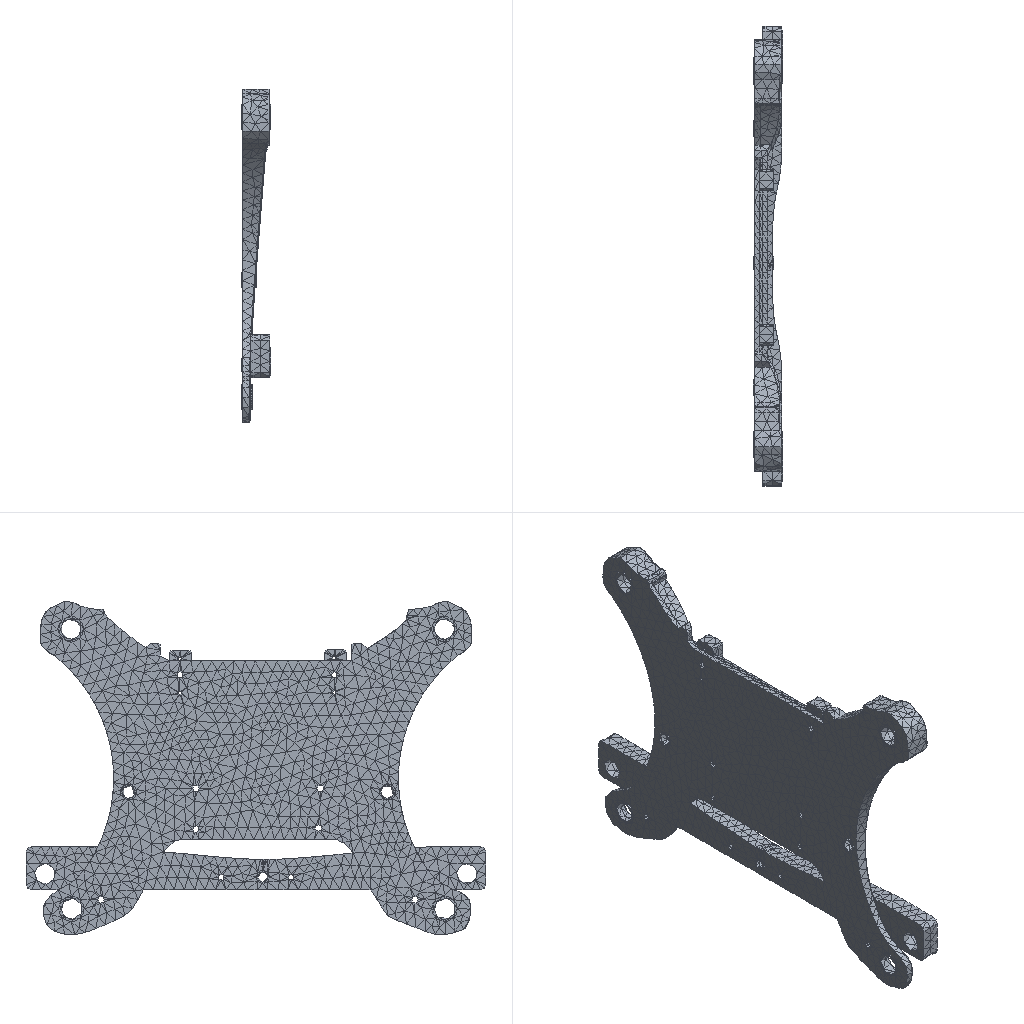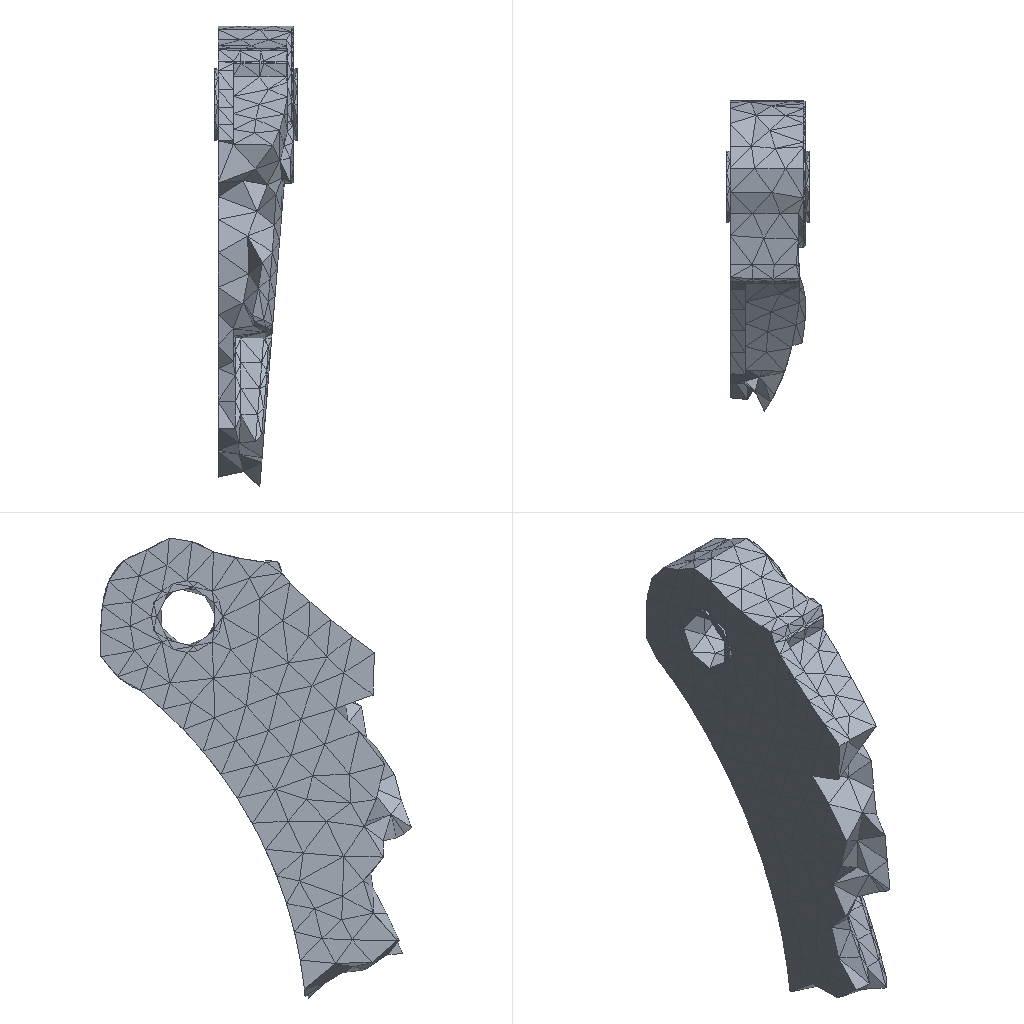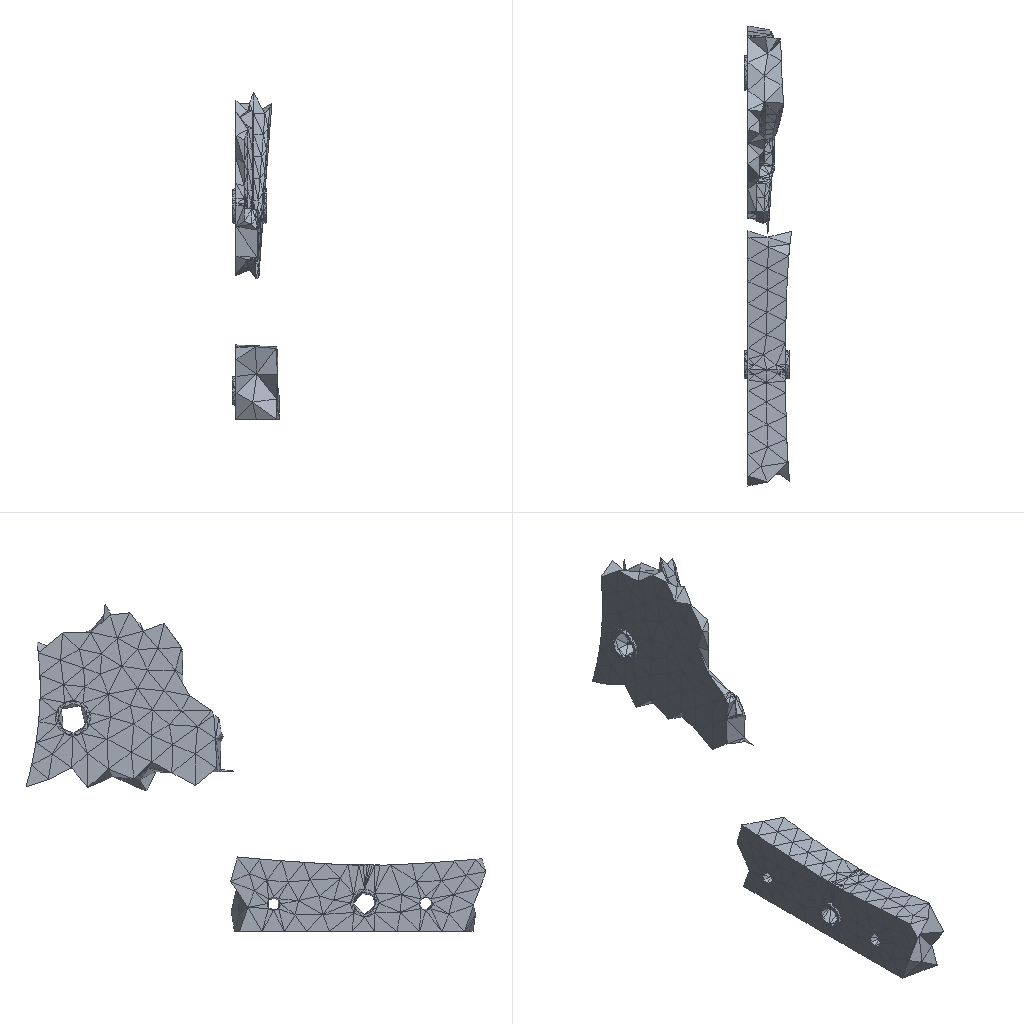Simulation study | ansys workbench
Set-up summary:
category,name,step,type,value,unit,region
solver,ansys_workbench
units,mm-N-s-tonne (MPa),,stated,"/units,MPA"
analysis,deck-1/LS1,,static
load_step,deck-1/LS1,deck-1/LS1,static,nsubst=1; time=1
analysis,deck-2/LS1,,modal,method=lanb; n_modes=6
load_step,deck-2/LS1,deck-2/LS1,modal
mesh,deck-1.dat,,nodes,30881
mesh,deck-1.dat,,elements,16295
element_type,SOLID187,,,16207,,deck-1.dat
element_type,SURF154,,,88,,deck-1.dat
mesh,deck-2.dat,,nodes,30881
mesh,deck-2.dat,,elements,16207
element_type,SOLID187,,,16207,,deck-2.dat
material,?,,E,210000,tonne s^-2 mm^-1
material,?,,nu,0.3
material,?,,density,7.85e-09,tonne mm^-3
load,Define Force Using Surface Effect Elements,deck-1/LS1,surface-effect pres face 1,0.105,,SURF154 #2
load,ACEL,deck-1/LS1,gravity (ACEL; gravity acts opposite),"29430 [dir=(-1, 0, 0)]",,all
bc,Fixed Supports,deck-1/model,fixed,[dofs=ALL],,_FIXEDSU
bc,Fixed Supports,deck-2/model,fixed,[dofs=ALL],,_FIXEDSU
named_set,_CM34_FIXEDSU,,node,341
named_set,_FIXEDSU,,node,341
named_set,_FIXEDSU,,node,341
Results summary:
result,analyses[0].index,,,1
result,analyses[0].system,,,SYS
result,analyses[0].deck,,,deck-1.dat
result,analyses[0].solve_status,,,completed
result,analyses[0].analysis_type,,,static
result,analyses[0].physics,,,mechanical
result,analyses[0].unit_system,,,"NMM: mm, ton, N, s, mV, mA, degC"
result,analyses[0].n_sets,,,1
result,analyses[0].load_steps[0].set,set=1,,1
result,analyses[0].load_steps[0].time_or_freq,set=1,,1
result,analyses[0].load_steps[0].max_displacement_magnitude,set=1,,0.02104
result,analyses[0].load_steps[0].max_von_mises_nodal,set=1,,7.878
result,analyses[0].load_steps[0].reaction_force_sum_xyz[1],set=1,,277.856
result,analyses[0].load_steps[0].reaction_force_sum_xyz[2],set=1,,-4.4836e-06
result,analyses[0].load_steps[0].reaction_force_sum_xyz[3],set=1,,6.94723e-06
result,analyses[1].index,,,2
result,analyses[1].system,,,SYS-1
result,analyses[1].deck,,,deck-2.dat
result,analyses[1].solve_status,,,completed
result,analyses[1].analysis_type,,,modal
result,analyses[1].physics,,,mechanical
result,analyses[1].unit_system,,,"NMM: mm, ton, N, s, mV, mA, degC"
result,analyses[1].n_sets,,,6
result,analyses[1].modal_frequencies_hz[1],,,253.849
result,analyses[1].modal_frequencies_hz[2],,,454.197
result,analyses[1].modal_frequencies_hz[3],,,502.307
result,analyses[1].modal_frequencies_hz[4],,,578.516
result,analyses[1].modal_frequencies_hz[5],,,664.088
result,analyses[1].modal_frequencies_hz[6],,,838.477